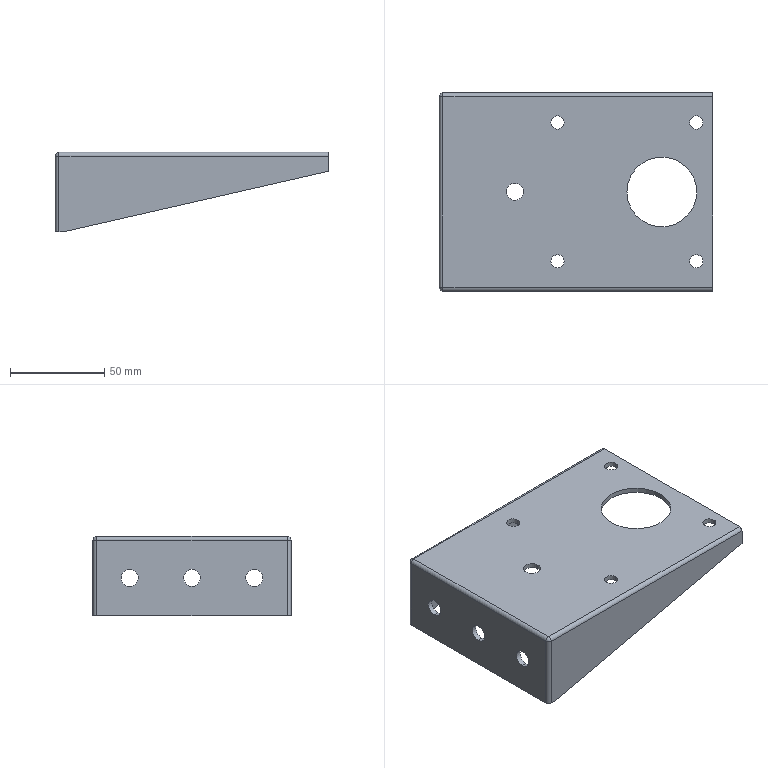Part | STEP file | 1.6米马达罩 | 1 solid | 40 faces | box 145 x 105 x 42 mm | volume 63685 mm3 | cylinder 26 | plane 12 | sphere 2 | commonest cylinder face diameters 7 x8 9 x8 4 x5 2 x3 37 x2
STEP:
#1=CARTESIAN_POINT('',(66.23,89.27,-2.6));
#2=VERTEX_POINT('',#1);
#3=CARTESIAN_POINT('',(59.23,89.27,-2.6));
#4=VERTEX_POINT('',#3);
#5=CARTESIAN_POINT('',(62.73,89.27,-2.6));
#6=DIRECTION('',(0.,0.,-1.));
#7=DIRECTION('',(-1.,0.,0.));
#8=AXIS2_PLACEMENT_3D('',#5,#6,#7);
#9=CIRCLE('',#8,3.5);
#10=EDGE_CURVE('',#2,#4,#9,.T.);
#11=ORIENTED_EDGE('',*,*,#10,.T.);
#12=CARTESIAN_POINT('',(59.23,89.27,0.));
#13=VERTEX_POINT('',#12);
#14=CARTESIAN_POINT('',(59.23,89.27,-10.));
#15=DIRECTION('',(0.,0.,1.));
#16=VECTOR('',#15,1000.);
#17=LINE('',#14,#16);
#18=EDGE_CURVE('',#4,#13,#17,.T.);
#19=ORIENTED_EDGE('',*,*,#18,.T.);
#20=CARTESIAN_POINT('',(66.23,89.27,0.));
#21=VERTEX_POINT('',#20);
#22=CARTESIAN_POINT('',(62.73,89.27,0.));
#23=DIRECTION('',(0.,0.,1.));
#24=DIRECTION('',(1.,0.,0.));
#25=AXIS2_PLACEMENT_3D('',#22,#23,#24);
#26=CIRCLE('',#25,3.5);
#27=EDGE_CURVE('',#13,#21,#26,.T.);
#28=ORIENTED_EDGE('',*,*,#27,.T.);
#29=CARTESIAN_POINT('',(66.23,89.27,-10.));
#30=DIRECTION('',(0.,0.,1.));
#31=VECTOR('',#30,1000.);
#32=LINE('',#29,#31);
#33=EDGE_CURVE('',#2,#21,#32,.T.);
#34=ORIENTED_EDGE('',*,*,#33,.F.);
#35=EDGE_LOOP('',(#11,#19,#28,#34));
#36=FACE_OUTER_BOUND('',#35,.T.);
#37=CARTESIAN_POINT('',(62.73,89.27,-10.));
#38=DIRECTION('',(0.,0.,1.));
#39=DIRECTION('',(1.,0.,0.));
#40=AXIS2_PLACEMENT_3D('',#37,#38,#39);
#41=CYLINDRICAL_SURFACE('',#40,3.5);
#42=ADVANCED_FACE('',(#36),#41,.F.);
#43=CARTESIAN_POINT('',(66.23,15.73,-2.6));
#44=VERTEX_POINT('',#43);
#45=CARTESIAN_POINT('',(59.23,15.73,-2.6));
#46=VERTEX_POINT('',#45);
#47=CARTESIAN_POINT('',(62.73,15.73,-2.6));
#48=DIRECTION('',(0.,0.,-1.));
#49=DIRECTION('',(-1.,0.,0.));
#50=AXIS2_PLACEMENT_3D('',#47,#48,#49);
#51=CIRCLE('',#50,3.5);
#52=EDGE_CURVE('',#44,#46,#51,.T.);
#53=ORIENTED_EDGE('',*,*,#52,.T.);
#54=CARTESIAN_POINT('',(59.23,15.73,0.));
#55=VERTEX_POINT('',#54);
#56=CARTESIAN_POINT('',(59.23,15.73,-10.));
#57=DIRECTION('',(0.,0.,1.));
#58=VECTOR('',#57,1000.);
#59=LINE('',#56,#58);
#60=EDGE_CURVE('',#46,#55,#59,.T.);
#61=ORIENTED_EDGE('',*,*,#60,.T.);
#62=CARTESIAN_POINT('',(66.23,15.73,0.));
#63=VERTEX_POINT('',#62);
#64=CARTESIAN_POINT('',(62.73,15.73,0.));
#65=DIRECTION('',(0.,0.,1.));
#66=DIRECTION('',(1.,0.,0.));
#67=AXIS2_PLACEMENT_3D('',#64,#65,#66);
#68=CIRCLE('',#67,3.5);
#69=EDGE_CURVE('',#55,#63,#68,.T.);
#70=ORIENTED_EDGE('',*,*,#69,.T.);
#71=CARTESIAN_POINT('',(66.23,15.73,-10.));
#72=DIRECTION('',(0.,0.,1.));
#73=VECTOR('',#72,1000.);
#74=LINE('',#71,#73);
#75=EDGE_CURVE('',#44,#63,#74,.T.);
#76=ORIENTED_EDGE('',*,*,#75,.F.);
#77=EDGE_LOOP('',(#53,#61,#70,#76));
#78=FACE_OUTER_BOUND('',#77,.T.);
#79=CARTESIAN_POINT('',(62.73,15.73,-10.));
#80=DIRECTION('',(0.,0.,1.));
#81=DIRECTION('',(1.,0.,0.));
#82=AXIS2_PLACEMENT_3D('',#79,#80,#81);
#83=CYLINDRICAL_SURFACE('',#82,3.5);
#84=ADVANCED_FACE('',(#78),#83,.F.);
#85=CARTESIAN_POINT('',(139.77,15.73,-2.6));
#86=VERTEX_POINT('',#85);
#87=CARTESIAN_POINT('',(132.77,15.73,-2.6));
#88=VERTEX_POINT('',#87);
#89=CARTESIAN_POINT('',(136.27,15.73,-2.6));
#90=DIRECTION('',(0.,0.,-1.));
#91=DIRECTION('',(-1.,0.,0.));
#92=AXIS2_PLACEMENT_3D('',#89,#90,#91);
#93=CIRCLE('',#92,3.5);
#94=EDGE_CURVE('',#86,#88,#93,.T.);
#95=ORIENTED_EDGE('',*,*,#94,.T.);
#96=CARTESIAN_POINT('',(132.77,15.73,0.));
#97=VERTEX_POINT('',#96);
#98=CARTESIAN_POINT('',(132.77,15.73,-10.));
#99=DIRECTION('',(0.,0.,1.));
#100=VECTOR('',#99,1000.);
#101=LINE('',#98,#100);
#102=EDGE_CURVE('',#88,#97,#101,.T.);
#103=ORIENTED_EDGE('',*,*,#102,.T.);
#104=CARTESIAN_POINT('',(139.77,15.73,0.));
#105=VERTEX_POINT('',#104);
#106=CARTESIAN_POINT('',(136.27,15.73,0.));
#107=DIRECTION('',(0.,0.,1.));
#108=DIRECTION('',(1.,0.,0.));
#109=AXIS2_PLACEMENT_3D('',#106,#107,#108);
#110=CIRCLE('',#109,3.5);
#111=EDGE_CURVE('',#97,#105,#110,.T.);
#112=ORIENTED_EDGE('',*,*,#111,.T.);
#113=CARTESIAN_POINT('',(139.77,15.73,-10.));
#114=DIRECTION('',(0.,0.,1.));
#115=VECTOR('',#114,1000.);
#116=LINE('',#113,#115);
#117=EDGE_CURVE('',#86,#105,#116,.T.);
#118=ORIENTED_EDGE('',*,*,#117,.F.);
#119=EDGE_LOOP('',(#95,#103,#112,#118));
#120=FACE_OUTER_BOUND('',#119,.T.);
#121=CARTESIAN_POINT('',(136.27,15.73,-10.));
#122=DIRECTION('',(0.,0.,1.));
#123=DIRECTION('',(1.,0.,0.));
#124=AXIS2_PLACEMENT_3D('',#121,#122,#123);
#125=CYLINDRICAL_SURFACE('',#124,3.5);
#126=ADVANCED_FACE('',(#120),#125,.F.);
#127=CARTESIAN_POINT('',(44.6,52.5,-2.6));
#128=VERTEX_POINT('',#127);
#129=CARTESIAN_POINT('',(35.6,52.5,-2.6));
#130=VERTEX_POINT('',#129);
#131=CARTESIAN_POINT('',(40.1,52.5,-2.6));
#132=DIRECTION('',(0.,0.,-1.));
#133=DIRECTION('',(-1.,0.,0.));
#134=AXIS2_PLACEMENT_3D('',#131,#132,#133);
#135=CIRCLE('',#134,4.5);
#136=EDGE_CURVE('',#128,#130,#135,.T.);
#137=ORIENTED_EDGE('',*,*,#136,.T.);
#138=CARTESIAN_POINT('',(35.6,52.5,0.));
#139=VERTEX_POINT('',#138);
#140=CARTESIAN_POINT('',(35.6,52.5,-10.));
#141=DIRECTION('',(0.,0.,1.));
#142=VECTOR('',#141,1000.);
#143=LINE('',#140,#142);
#144=EDGE_CURVE('',#130,#139,#143,.T.);
#145=ORIENTED_EDGE('',*,*,#144,.T.);
#146=CARTESIAN_POINT('',(44.6,52.5,0.));
#147=VERTEX_POINT('',#146);
#148=CARTESIAN_POINT('',(40.1,52.5,0.));
#149=DIRECTION('',(0.,0.,1.));
#150=DIRECTION('',(1.,0.,0.));
#151=AXIS2_PLACEMENT_3D('',#148,#149,#150);
#152=CIRCLE('',#151,4.5);
#153=EDGE_CURVE('',#139,#147,#152,.T.);
#154=ORIENTED_EDGE('',*,*,#153,.T.);
#155=CARTESIAN_POINT('',(44.6,52.5,-10.));
#156=DIRECTION('',(0.,0.,1.));
#157=VECTOR('',#156,1000.);
#158=LINE('',#155,#157);
#159=EDGE_CURVE('',#128,#147,#158,.T.);
#160=ORIENTED_EDGE('',*,*,#159,.F.);
#161=EDGE_LOOP('',(#137,#145,#154,#160));
#162=FACE_OUTER_BOUND('',#161,.T.);
#163=CARTESIAN_POINT('',(40.1,52.5,-10.));
#164=DIRECTION('',(0.,0.,1.));
#165=DIRECTION('',(1.,0.,0.));
#166=AXIS2_PLACEMENT_3D('',#163,#164,#165);
#167=CYLINDRICAL_SURFACE('',#166,4.5);
#168=ADVANCED_FACE('',(#162),#167,.F.);
#169=CARTESIAN_POINT('',(139.77,89.27,-2.6));
#170=VERTEX_POINT('',#169);
#171=CARTESIAN_POINT('',(132.77,89.27,-2.6));
#172=VERTEX_POINT('',#171);
#173=CARTESIAN_POINT('',(136.27,89.27,-2.6));
#174=DIRECTION('',(0.,0.,-1.));
#175=DIRECTION('',(-1.,0.,0.));
#176=AXIS2_PLACEMENT_3D('',#173,#174,#175);
#177=CIRCLE('',#176,3.5);
#178=EDGE_CURVE('',#170,#172,#177,.T.);
#179=ORIENTED_EDGE('',*,*,#178,.T.);
#180=CARTESIAN_POINT('',(132.77,89.27,0.));
#181=VERTEX_POINT('',#180);
#182=CARTESIAN_POINT('',(132.77,89.27,-10.));
#183=DIRECTION('',(0.,0.,1.));
#184=VECTOR('',#183,1000.);
#185=LINE('',#182,#184);
#186=EDGE_CURVE('',#172,#181,#185,.T.);
#187=ORIENTED_EDGE('',*,*,#186,.T.);
#188=CARTESIAN_POINT('',(139.77,89.27,0.));
#189=VERTEX_POINT('',#188);
#190=CARTESIAN_POINT('',(136.27,89.27,0.));
#191=DIRECTION('',(0.,0.,1.));
#192=DIRECTION('',(1.,0.,0.));
#193=AXIS2_PLACEMENT_3D('',#190,#191,#192);
#194=CIRCLE('',#193,3.5);
#195=EDGE_CURVE('',#181,#189,#194,.T.);
#196=ORIENTED_EDGE('',*,*,#195,.T.);
#197=CARTESIAN_POINT('',(139.77,89.27,-10.));
#198=DIRECTION('',(0.,0.,1.));
#199=VECTOR('',#198,1000.);
#200=LINE('',#197,#199);
#201=EDGE_CURVE('',#170,#189,#200,.T.);
#202=ORIENTED_EDGE('',*,*,#201,.F.);
#203=EDGE_LOOP('',(#179,#187,#196,#202));
#204=FACE_OUTER_BOUND('',#203,.T.);
#205=CARTESIAN_POINT('',(136.27,89.27,-10.));
#206=DIRECTION('',(0.,0.,1.));
#207=DIRECTION('',(1.,0.,0.));
#208=AXIS2_PLACEMENT_3D('',#205,#206,#207);
#209=CYLINDRICAL_SURFACE('',#208,3.5);
#210=ADVANCED_FACE('',(#204),#209,.F.);
#211=CARTESIAN_POINT('',(136.5,52.5,-2.6));
#212=VERTEX_POINT('',#211);
#213=CARTESIAN_POINT('',(99.5,52.5,-2.6));
#214=VERTEX_POINT('',#213);
#215=CARTESIAN_POINT('',(118.,52.5,-2.6));
#216=DIRECTION('',(0.,0.,-1.));
#217=DIRECTION('',(-1.,0.,0.));
#218=AXIS2_PLACEMENT_3D('',#215,#216,#217);
#219=CIRCLE('',#218,18.5);
#220=EDGE_CURVE('',#212,#214,#219,.T.);
#221=ORIENTED_EDGE('',*,*,#220,.T.);
#222=CARTESIAN_POINT('',(99.5,52.5,0.));
#223=VERTEX_POINT('',#222);
#224=CARTESIAN_POINT('',(99.5,52.5,-10.));
#225=DIRECTION('',(0.,0.,1.));
#226=VECTOR('',#225,1000.);
#227=LINE('',#224,#226);
#228=EDGE_CURVE('',#214,#223,#227,.T.);
#229=ORIENTED_EDGE('',*,*,#228,.T.);
#230=CARTESIAN_POINT('',(136.5,52.5,0.));
#231=VERTEX_POINT('',#230);
#232=CARTESIAN_POINT('',(118.,52.5,0.));
#233=DIRECTION('',(0.,0.,1.));
#234=DIRECTION('',(1.,0.,0.));
#235=AXIS2_PLACEMENT_3D('',#232,#233,#234);
#236=CIRCLE('',#235,18.5);
#237=EDGE_CURVE('',#223,#231,#236,.T.);
#238=ORIENTED_EDGE('',*,*,#237,.T.);
#239=CARTESIAN_POINT('',(136.5,52.5,-10.));
#240=DIRECTION('',(0.,0.,1.));
#241=VECTOR('',#240,1000.);
#242=LINE('',#239,#241);
#243=EDGE_CURVE('',#212,#231,#242,.T.);
#244=ORIENTED_EDGE('',*,*,#243,.F.);
#245=EDGE_LOOP('',(#221,#229,#238,#244));
#246=FACE_OUTER_BOUND('',#245,.T.);
#247=CARTESIAN_POINT('',(118.,52.5,-10.));
#248=DIRECTION('',(0.,0.,1.));
#249=DIRECTION('',(1.,0.,0.));
#250=AXIS2_PLACEMENT_3D('',#247,#248,#249);
#251=CYLINDRICAL_SURFACE('',#250,18.5);
#252=ADVANCED_FACE('',(#246),#251,.F.);
#253=CARTESIAN_POINT('',(2.6,19.5,-17.5));
#254=VERTEX_POINT('',#253);
#255=CARTESIAN_POINT('',(2.6,19.5,-26.5));
#256=VERTEX_POINT('',#255);
#257=CARTESIAN_POINT('',(2.6,19.5,-22.));
#258=DIRECTION('',(1.,0.,0.));
#259=DIRECTION('',(0.,0.,-1.));
#260=AXIS2_PLACEMENT_3D('',#257,#258,#259);
#261=CIRCLE('',#260,4.5);
#262=EDGE_CURVE('',#254,#256,#261,.T.);
#263=ORIENTED_EDGE('',*,*,#262,.T.);
#264=CARTESIAN_POINT('',(0.,19.5,-26.5));
#265=VERTEX_POINT('',#264);
#266=CARTESIAN_POINT('',(10.,19.5,-26.5));
#267=DIRECTION('',(-1.,0.,0.));
#268=VECTOR('',#267,1000.);
#269=LINE('',#266,#268);
#270=EDGE_CURVE('',#256,#265,#269,.T.);
#271=ORIENTED_EDGE('',*,*,#270,.T.);
#272=CARTESIAN_POINT('',(0.,19.5,-17.5));
#273=VERTEX_POINT('',#272);
#274=CARTESIAN_POINT('',(0.,19.5,-22.));
#275=DIRECTION('',(-1.,0.,0.));
#276=DIRECTION('',(0.,0.,1.));
#277=AXIS2_PLACEMENT_3D('',#274,#275,#276);
#278=CIRCLE('',#277,4.5);
#279=EDGE_CURVE('',#265,#273,#278,.T.);
#280=ORIENTED_EDGE('',*,*,#279,.T.);
#281=CARTESIAN_POINT('',(10.,19.5,-17.5));
#282=DIRECTION('',(-1.,0.,0.));
#283=VECTOR('',#282,1000.);
#284=LINE('',#281,#283);
#285=EDGE_CURVE('',#254,#273,#284,.T.);
#286=ORIENTED_EDGE('',*,*,#285,.F.);
#287=EDGE_LOOP('',(#263,#271,#280,#286));
#288=FACE_OUTER_BOUND('',#287,.T.);
#289=CARTESIAN_POINT('',(10.,19.5,-22.));
#290=DIRECTION('',(-1.,0.,0.));
#291=DIRECTION('',(0.,0.,1.));
#292=AXIS2_PLACEMENT_3D('',#289,#290,#291);
#293=CYLINDRICAL_SURFACE('',#292,4.5);
#294=ADVANCED_FACE('',(#288),#293,.F.);
#295=CARTESIAN_POINT('',(2.6,85.5,-17.5));
#296=VERTEX_POINT('',#295);
#297=CARTESIAN_POINT('',(2.6,85.5,-26.5));
#298=VERTEX_POINT('',#297);
#299=CARTESIAN_POINT('',(2.6,85.5,-22.));
#300=DIRECTION('',(1.,0.,0.));
#301=DIRECTION('',(0.,0.,-1.));
#302=AXIS2_PLACEMENT_3D('',#299,#300,#301);
#303=CIRCLE('',#302,4.5);
#304=EDGE_CURVE('',#296,#298,#303,.T.);
#305=ORIENTED_EDGE('',*,*,#304,.T.);
#306=CARTESIAN_POINT('',(0.,85.5,-26.5));
#307=VERTEX_POINT('',#306);
#308=CARTESIAN_POINT('',(10.,85.5,-26.5));
#309=DIRECTION('',(-1.,0.,0.));
#310=VECTOR('',#309,1000.);
#311=LINE('',#308,#310);
#312=EDGE_CURVE('',#298,#307,#311,.T.);
#313=ORIENTED_EDGE('',*,*,#312,.T.);
#314=CARTESIAN_POINT('',(0.,85.5,-17.5));
#315=VERTEX_POINT('',#314);
#316=CARTESIAN_POINT('',(0.,85.5,-22.));
#317=DIRECTION('',(-1.,0.,0.));
#318=DIRECTION('',(0.,0.,1.));
#319=AXIS2_PLACEMENT_3D('',#316,#317,#318);
#320=CIRCLE('',#319,4.5);
#321=EDGE_CURVE('',#307,#315,#320,.T.);
#322=ORIENTED_EDGE('',*,*,#321,.T.);
#323=CARTESIAN_POINT('',(10.,85.5,-17.5));
#324=DIRECTION('',(-1.,0.,0.));
#325=VECTOR('',#324,1000.);
#326=LINE('',#323,#325);
#327=EDGE_CURVE('',#296,#315,#326,.T.);
#328=ORIENTED_EDGE('',*,*,#327,.F.);
#329=EDGE_LOOP('',(#305,#313,#322,#328));
#330=FACE_OUTER_BOUND('',#329,.T.);
#331=CARTESIAN_POINT('',(10.,85.5,-22.));
#332=DIRECTION('',(-1.,0.,0.));
#333=DIRECTION('',(0.,0.,1.));
#334=AXIS2_PLACEMENT_3D('',#331,#332,#333);
#335=CYLINDRICAL_SURFACE('',#334,4.5);
#336=ADVANCED_FACE('',(#330),#335,.F.);
#337=CARTESIAN_POINT('',(2.6,52.5,-17.5));
#338=VERTEX_POINT('',#337);
#339=CARTESIAN_POINT('',(2.6,52.5,-26.5));
#340=VERTEX_POINT('',#339);
#341=CARTESIAN_POINT('',(2.6,52.5,-22.));
#342=DIRECTION('',(1.,0.,0.));
#343=DIRECTION('',(0.,0.,-1.));
#344=AXIS2_PLACEMENT_3D('',#341,#342,#343);
#345=CIRCLE('',#344,4.5);
#346=EDGE_CURVE('',#338,#340,#345,.T.);
#347=ORIENTED_EDGE('',*,*,#346,.T.);
#348=CARTESIAN_POINT('',(0.,52.5,-26.5));
#349=VERTEX_POINT('',#348);
#350=CARTESIAN_POINT('',(10.,52.5,-26.5));
#351=DIRECTION('',(-1.,0.,0.));
#352=VECTOR('',#351,1000.);
#353=LINE('',#350,#352);
#354=EDGE_CURVE('',#340,#349,#353,.T.);
#355=ORIENTED_EDGE('',*,*,#354,.T.);
#356=CARTESIAN_POINT('',(0.,52.5,-17.5));
#357=VERTEX_POINT('',#356);
#358=CARTESIAN_POINT('',(0.,52.5,-22.));
#359=DIRECTION('',(-1.,0.,0.));
#360=DIRECTION('',(0.,0.,1.));
#361=AXIS2_PLACEMENT_3D('',#358,#359,#360);
#362=CIRCLE('',#361,4.5);
#363=EDGE_CURVE('',#349,#357,#362,.T.);
#364=ORIENTED_EDGE('',*,*,#363,.T.);
#365=CARTESIAN_POINT('',(10.,52.5,-17.5));
#366=DIRECTION('',(-1.,0.,0.));
#367=VECTOR('',#366,1000.);
#368=LINE('',#365,#367);
#369=EDGE_CURVE('',#338,#357,#368,.T.);
#370=ORIENTED_EDGE('',*,*,#369,.F.);
#371=EDGE_LOOP('',(#347,#355,#364,#370));
#372=FACE_OUTER_BOUND('',#371,.T.);
#373=CARTESIAN_POINT('',(10.,52.5,-22.));
#374=DIRECTION('',(-1.,0.,0.));
#375=DIRECTION('',(0.,0.,1.));
#376=AXIS2_PLACEMENT_3D('',#373,#374,#375);
#377=CYLINDRICAL_SURFACE('',#376,4.5);
#378=ADVANCED_FACE('',(#372),#377,.F.);
#379=CARTESIAN_POINT('',(145.,103.,0.));
#380=VERTEX_POINT('',#379);
#381=CARTESIAN_POINT('',(145.,2.,0.));
#382=VERTEX_POINT('',#381);
#383=CARTESIAN_POINT('',(145.,105.,0.));
#384=DIRECTION('',(0.,-1.,0.));
#385=VECTOR('',#384,1000.);
#386=LINE('',#383,#385);
#387=EDGE_CURVE('',#380,#382,#386,.T.);
#388=ORIENTED_EDGE('',*,*,#387,.T.);
#389=CARTESIAN_POINT('',(145.,0.,-2.));
#390=VERTEX_POINT('',#389);
#391=CARTESIAN_POINT('',(145.,2.,-2.));
#392=DIRECTION('',(1.,0.,0.));
#393=DIRECTION('',(0.,0.,1.));
#394=AXIS2_PLACEMENT_3D('',#391,#392,#393);
#395=CIRCLE('',#394,2.);
#396=EDGE_CURVE('',#382,#390,#395,.T.);
#397=ORIENTED_EDGE('',*,*,#396,.T.);
#398=CARTESIAN_POINT('',(145.,0.,-10.));
#399=VERTEX_POINT('',#398);
#400=CARTESIAN_POINT('',(145.,0.,-10.));
#401=DIRECTION('',(0.,0.,-1.));
#402=VECTOR('',#401,1000.);
#403=LINE('',#400,#402);
#404=EDGE_CURVE('',#390,#399,#403,.T.);
#405=ORIENTED_EDGE('',*,*,#404,.T.);
#406=CARTESIAN_POINT('',(145.,2.6,-10.));
#407=VERTEX_POINT('',#406);
#408=CARTESIAN_POINT('',(145.,105.,-10.));
#409=DIRECTION('',(0.,-1.,0.));
#410=VECTOR('',#409,1000.);
#411=LINE('',#408,#410);
#412=EDGE_CURVE('',#407,#399,#411,.T.);
#413=ORIENTED_EDGE('',*,*,#412,.F.);
#414=CARTESIAN_POINT('',(145.,2.6,-3.6));
#415=VERTEX_POINT('',#414);
#416=CARTESIAN_POINT('',(145.,2.6,0.));
#417=DIRECTION('',(0.,0.,-1.));
#418=VECTOR('',#417,1000.);
#419=LINE('',#416,#418);
#420=EDGE_CURVE('',#415,#407,#419,.T.);
#421=ORIENTED_EDGE('',*,*,#420,.F.);
#422=CARTESIAN_POINT('',(145.,3.6,-2.6));
#423=VERTEX_POINT('',#422);
#424=CARTESIAN_POINT('',(145.,3.6,-3.6));
#425=DIRECTION('',(-1.,0.,0.));
#426=DIRECTION('',(0.,0.,1.));
#427=AXIS2_PLACEMENT_3D('',#424,#425,#426);
#428=CIRCLE('',#427,1.);
#429=EDGE_CURVE('',#415,#423,#428,.T.);
#430=ORIENTED_EDGE('',*,*,#429,.T.);
#431=CARTESIAN_POINT('',(145.,101.4,-2.6));
#432=VERTEX_POINT('',#431);
#433=CARTESIAN_POINT('',(145.,105.,-2.6));
#434=DIRECTION('',(0.,-1.,0.));
#435=VECTOR('',#434,1000.);
#436=LINE('',#433,#435);
#437=EDGE_CURVE('',#432,#423,#436,.T.);
#438=ORIENTED_EDGE('',*,*,#437,.F.);
#439=CARTESIAN_POINT('',(145.,102.4,-3.6));
#440=VERTEX_POINT('',#439);
#441=CARTESIAN_POINT('',(145.,101.4,-3.6));
#442=DIRECTION('',(-1.,0.,0.));
#443=DIRECTION('',(0.,0.,1.));
#444=AXIS2_PLACEMENT_3D('',#441,#442,#443);
#445=CIRCLE('',#444,1.);
#446=EDGE_CURVE('',#432,#440,#445,.T.);
#447=ORIENTED_EDGE('',*,*,#446,.T.);
#448=CARTESIAN_POINT('',(145.,102.4,-10.));
#449=VERTEX_POINT('',#448);
#450=CARTESIAN_POINT('',(145.,102.4,0.));
#451=DIRECTION('',(0.,0.,-1.));
#452=VECTOR('',#451,1000.);
#453=LINE('',#450,#452);
#454=EDGE_CURVE('',#440,#449,#453,.T.);
#455=ORIENTED_EDGE('',*,*,#454,.T.);
#456=CARTESIAN_POINT('',(145.,105.,-10.));
#457=VERTEX_POINT('',#456);
#458=CARTESIAN_POINT('',(145.,105.,-10.));
#459=DIRECTION('',(0.,-1.,0.));
#460=VECTOR('',#459,1000.);
#461=LINE('',#458,#460);
#462=EDGE_CURVE('',#457,#449,#461,.T.);
#463=ORIENTED_EDGE('',*,*,#462,.F.);
#464=CARTESIAN_POINT('',(145.,105.,-2.));
#465=VERTEX_POINT('',#464);
#466=CARTESIAN_POINT('',(145.,105.,-10.));
#467=DIRECTION('',(0.,0.,-1.));
#468=VECTOR('',#467,1000.);
#469=LINE('',#466,#468);
#470=EDGE_CURVE('',#465,#457,#469,.T.);
#471=ORIENTED_EDGE('',*,*,#470,.F.);
#472=CARTESIAN_POINT('',(145.,103.,-2.));
#473=DIRECTION('',(1.,0.,0.));
#474=DIRECTION('',(0.,0.,1.));
#475=AXIS2_PLACEMENT_3D('',#472,#473,#474);
#476=CIRCLE('',#475,2.);
#477=EDGE_CURVE('',#465,#380,#476,.T.);
#478=ORIENTED_EDGE('',*,*,#477,.T.);
#479=EDGE_LOOP('',(#388,#397,#405,#413,#421,#430,#438,#447,#455,#463,#471,#478));
#480=FACE_OUTER_BOUND('',#479,.T.);
#481=CARTESIAN_POINT('',(145.,105.,-10.));
#482=DIRECTION('',(-1.,0.,0.));
#483=DIRECTION('',(0.,0.,1.));
#484=AXIS2_PLACEMENT_3D('',#481,#482,#483);
#485=PLANE('',#484);
#486=ADVANCED_FACE('',(#480),#485,.F.);
#487=CARTESIAN_POINT('',(5.,2.6,-42.));
#488=VERTEX_POINT('',#487);
#489=CARTESIAN_POINT('',(9.372,2.6,-41.001));
#490=DIRECTION('',(-0.9749,0.,-0.2228));
#491=VECTOR('',#490,1000.);
#492=LINE('',#489,#491);
#493=EDGE_CURVE('',#407,#488,#492,.T.);
#494=ORIENTED_EDGE('',*,*,#493,.F.);
#495=ORIENTED_EDGE('',*,*,#412,.T.);
#496=CARTESIAN_POINT('',(5.,0.,-42.));
#497=VERTEX_POINT('',#496);
#498=CARTESIAN_POINT('',(5.,0.,-42.));
#499=DIRECTION('',(-0.9749,0.,-0.2228));
#500=VECTOR('',#499,1000.);
#501=LINE('',#498,#500);
#502=EDGE_CURVE('',#399,#497,#501,.T.);
#503=ORIENTED_EDGE('',*,*,#502,.T.);
#504=CARTESIAN_POINT('',(5.,105.,-42.));
#505=DIRECTION('',(0.,-1.,0.));
#506=VECTOR('',#505,1000.);
#507=LINE('',#504,#506);
#508=EDGE_CURVE('',#488,#497,#507,.T.);
#509=ORIENTED_EDGE('',*,*,#508,.F.);
#510=EDGE_LOOP('',(#494,#495,#503,#509));
#511=FACE_OUTER_BOUND('',#510,.T.);
#512=CARTESIAN_POINT('',(5.,105.,-42.));
#513=DIRECTION('',(-0.2228,0.,0.9749));
#514=DIRECTION('',(0.9749,0.,0.2228));
#515=AXIS2_PLACEMENT_3D('',#512,#513,#514);
#516=PLANE('',#515);
#517=ADVANCED_FACE('',(#511),#516,.F.);
#518=CARTESIAN_POINT('',(2.,0.,-42.));
#519=VERTEX_POINT('',#518);
#520=CARTESIAN_POINT('',(0.,0.,-42.));
#521=DIRECTION('',(-1.,0.,0.));
#522=VECTOR('',#521,1000.);
#523=LINE('',#520,#522);
#524=EDGE_CURVE('',#497,#519,#523,.T.);
#525=ORIENTED_EDGE('',*,*,#524,.T.);
#526=CARTESIAN_POINT('',(0.,2.,-42.));
#527=VERTEX_POINT('',#526);
#528=CARTESIAN_POINT('',(2.,2.,-42.));
#529=DIRECTION('',(0.,0.,-1.));
#530=DIRECTION('',(1.,0.,0.));
#531=AXIS2_PLACEMENT_3D('',#528,#529,#530);
#532=CIRCLE('',#531,2.);
#533=EDGE_CURVE('',#519,#527,#532,.T.);
#534=ORIENTED_EDGE('',*,*,#533,.T.);
#535=CARTESIAN_POINT('',(0.,103.,-42.));
#536=VERTEX_POINT('',#535);
#537=CARTESIAN_POINT('',(0.,105.,-42.));
#538=DIRECTION('',(0.,-1.,0.));
#539=VECTOR('',#538,1000.);
#540=LINE('',#537,#539);
#541=EDGE_CURVE('',#536,#527,#540,.T.);
#542=ORIENTED_EDGE('',*,*,#541,.F.);
#543=CARTESIAN_POINT('',(2.,105.,-42.));
#544=VERTEX_POINT('',#543);
#545=CARTESIAN_POINT('',(2.,103.,-42.));
#546=DIRECTION('',(0.,0.,-1.));
#547=DIRECTION('',(1.,0.,0.));
#548=AXIS2_PLACEMENT_3D('',#545,#546,#547);
#549=CIRCLE('',#548,2.);
#550=EDGE_CURVE('',#536,#544,#549,.T.);
#551=ORIENTED_EDGE('',*,*,#550,.T.);
#552=CARTESIAN_POINT('',(5.,105.,-42.));
#553=VERTEX_POINT('',#552);
#554=CARTESIAN_POINT('',(0.,105.,-42.));
#555=DIRECTION('',(-1.,0.,0.));
#556=VECTOR('',#555,1000.);
#557=LINE('',#554,#556);
#558=EDGE_CURVE('',#553,#544,#557,.T.);
#559=ORIENTED_EDGE('',*,*,#558,.F.);
#560=CARTESIAN_POINT('',(5.,102.4,-42.));
#561=VERTEX_POINT('',#560);
#562=CARTESIAN_POINT('',(5.,105.,-42.));
#563=DIRECTION('',(0.,-1.,0.));
#564=VECTOR('',#563,1000.);
#565=LINE('',#562,#564);
#566=EDGE_CURVE('',#553,#561,#565,.T.);
#567=ORIENTED_EDGE('',*,*,#566,.T.);
#568=CARTESIAN_POINT('',(2.6,102.4,-42.));
#569=VERTEX_POINT('',#568);
#570=CARTESIAN_POINT('',(0.,102.4,-42.));
#571=DIRECTION('',(-1.,0.,0.));
#572=VECTOR('',#571,1000.);
#573=LINE('',#570,#572);
#574=EDGE_CURVE('',#561,#569,#573,.T.);
#575=ORIENTED_EDGE('',*,*,#574,.T.);
#576=CARTESIAN_POINT('',(2.6,2.6,-42.));
#577=VERTEX_POINT('',#576);
#578=CARTESIAN_POINT('',(2.6,105.,-42.));
#579=DIRECTION('',(0.,-1.,0.));
#580=VECTOR('',#579,1000.);
#581=LINE('',#578,#580);
#582=EDGE_CURVE('',#569,#577,#581,.T.);
#583=ORIENTED_EDGE('',*,*,#582,.T.);
#584=CARTESIAN_POINT('',(0.,2.6,-42.));
#585=DIRECTION('',(-1.,0.,0.));
#586=VECTOR('',#585,1000.);
#587=LINE('',#584,#586);
#588=EDGE_CURVE('',#488,#577,#587,.T.);
#589=ORIENTED_EDGE('',*,*,#588,.F.);
#590=ORIENTED_EDGE('',*,*,#508,.T.);
#591=EDGE_LOOP('',(#525,#534,#542,#551,#559,#567,#575,#583,#589,#590));
#592=FACE_OUTER_BOUND('',#591,.T.);
#593=CARTESIAN_POINT('',(0.,105.,-42.));
#594=DIRECTION('',(0.,0.,1.));
#595=DIRECTION('',(1.,0.,0.));
#596=AXIS2_PLACEMENT_3D('',#593,#594,#595);
#597=PLANE('',#596);
#598=ADVANCED_FACE('',(#592),#597,.F.);
#599=CARTESIAN_POINT('',(62.73,89.27,0.));
#600=DIRECTION('',(0.,0.,1.));
#601=DIRECTION('',(1.,0.,0.));
#602=AXIS2_PLACEMENT_3D('',#599,#600,#601);
#603=CIRCLE('',#602,3.5);
#604=EDGE_CURVE('',#21,#13,#603,.T.);
#605=ORIENTED_EDGE('',*,*,#604,.F.);
#606=ORIENTED_EDGE('',*,*,#27,.F.);
#607=EDGE_LOOP('',(#605,#606));
#608=FACE_BOUND('',#607,.T.);
#609=CARTESIAN_POINT('',(62.73,15.73,0.));
#610=DIRECTION('',(0.,0.,1.));
#611=DIRECTION('',(1.,0.,0.));
#612=AXIS2_PLACEMENT_3D('',#609,#610,#611);
#613=CIRCLE('',#612,3.5);
#614=EDGE_CURVE('',#63,#55,#613,.T.);
#615=ORIENTED_EDGE('',*,*,#614,.F.);
#616=ORIENTED_EDGE('',*,*,#69,.F.);
#617=EDGE_LOOP('',(#615,#616));
#618=FACE_BOUND('',#617,.T.);
#619=CARTESIAN_POINT('',(136.27,15.73,0.));
#620=DIRECTION('',(0.,0.,1.));
#621=DIRECTION('',(1.,0.,0.));
#622=AXIS2_PLACEMENT_3D('',#619,#620,#621);
#623=CIRCLE('',#622,3.5);
#624=EDGE_CURVE('',#105,#97,#623,.T.);
#625=ORIENTED_EDGE('',*,*,#624,.F.);
#626=ORIENTED_EDGE('',*,*,#111,.F.);
#627=EDGE_LOOP('',(#625,#626));
#628=FACE_BOUND('',#627,.T.);
#629=CARTESIAN_POINT('',(40.1,52.5,0.));
#630=DIRECTION('',(0.,0.,1.));
#631=DIRECTION('',(1.,0.,0.));
#632=AXIS2_PLACEMENT_3D('',#629,#630,#631);
#633=CIRCLE('',#632,4.5);
#634=EDGE_CURVE('',#147,#139,#633,.T.);
#635=ORIENTED_EDGE('',*,*,#634,.F.);
#636=ORIENTED_EDGE('',*,*,#153,.F.);
#637=EDGE_LOOP('',(#635,#636));
#638=FACE_BOUND('',#637,.T.);
#639=CARTESIAN_POINT('',(136.27,89.27,0.));
#640=DIRECTION('',(0.,0.,1.));
#641=DIRECTION('',(1.,0.,0.));
#642=AXIS2_PLACEMENT_3D('',#639,#640,#641);
#643=CIRCLE('',#642,3.5);
#644=EDGE_CURVE('',#189,#181,#643,.T.);
#645=ORIENTED_EDGE('',*,*,#644,.F.);
#646=ORIENTED_EDGE('',*,*,#195,.F.);
#647=EDGE_LOOP('',(#645,#646));
#648=FACE_BOUND('',#647,.T.);
#649=CARTESIAN_POINT('',(118.,52.5,0.));
#650=DIRECTION('',(0.,0.,1.));
#651=DIRECTION('',(1.,0.,0.));
#652=AXIS2_PLACEMENT_3D('',#649,#650,#651);
#653=CIRCLE('',#652,18.5);
#654=EDGE_CURVE('',#231,#223,#653,.T.);
#655=ORIENTED_EDGE('',*,*,#654,.F.);
#656=ORIENTED_EDGE('',*,*,#237,.F.);
#657=EDGE_LOOP('',(#655,#656));
#658=FACE_BOUND('',#657,.T.);
#659=CARTESIAN_POINT('',(2.,103.,0.));
#660=VERTEX_POINT('',#659);
#661=CARTESIAN_POINT('',(2.,2.,0.));
#662=VERTEX_POINT('',#661);
#663=CARTESIAN_POINT('',(2.,105.,0.));
#664=DIRECTION('',(0.,-1.,0.));
#665=VECTOR('',#664,1000.);
#666=LINE('',#663,#665);
#667=EDGE_CURVE('',#660,#662,#666,.T.);
#668=ORIENTED_EDGE('',*,*,#667,.T.);
#669=CARTESIAN_POINT('',(145.,2.,0.));
#670=DIRECTION('',(1.,0.,0.));
#671=VECTOR('',#670,1000.);
#672=LINE('',#669,#671);
#673=EDGE_CURVE('',#662,#382,#672,.T.);
#674=ORIENTED_EDGE('',*,*,#673,.T.);
#675=ORIENTED_EDGE('',*,*,#387,.F.);
#676=CARTESIAN_POINT('',(145.,103.,0.));
#677=DIRECTION('',(-1.,0.,0.));
#678=VECTOR('',#677,1000.);
#679=LINE('',#676,#678);
#680=EDGE_CURVE('',#380,#660,#679,.T.);
#681=ORIENTED_EDGE('',*,*,#680,.T.);
#682=EDGE_LOOP('',(#668,#674,#675,#681));
#683=FACE_OUTER_BOUND('',#682,.T.);
#684=CARTESIAN_POINT('',(145.,105.,0.));
#685=DIRECTION('',(0.,0.,-1.));
#686=DIRECTION('',(-1.,0.,0.));
#687=AXIS2_PLACEMENT_3D('',#684,#685,#686);
#688=PLANE('',#687);
#689=ADVANCED_FACE('',(#608,#618,#628,#638,#648,#658,#683),#688,.F.);
#690=ORIENTED_EDGE('',*,*,#462,.T.);
#691=CARTESIAN_POINT('',(9.372,102.4,-41.001));
#692=DIRECTION('',(-0.9749,0.,-0.2228));
#693=VECTOR('',#692,1000.);
#694=LINE('',#691,#693);
#695=EDGE_CURVE('',#449,#561,#694,.T.);
#696=ORIENTED_EDGE('',*,*,#695,.T.);
#697=ORIENTED_EDGE('',*,*,#566,.F.);
#698=CARTESIAN_POINT('',(5.,105.,-42.));
#699=DIRECTION('',(-0.9749,0.,-0.2228));
#700=VECTOR('',#699,1000.);
#701=LINE('',#698,#700);
#702=EDGE_CURVE('',#457,#553,#701,.T.);
#703=ORIENTED_EDGE('',*,*,#702,.F.);
#704=EDGE_LOOP('',(#690,#696,#697,#703));
#705=FACE_OUTER_BOUND('',#704,.T.);
#706=CARTESIAN_POINT('',(5.,105.,-42.));
#707=DIRECTION('',(-0.2228,0.,0.9749));
#708=DIRECTION('',(0.9749,0.,0.2228));
#709=AXIS2_PLACEMENT_3D('',#706,#707,#708);
#710=PLANE('',#709);
#711=ADVANCED_FACE('',(#705),#710,.F.);
#712=CARTESIAN_POINT('',(0.,19.5,-22.));
#713=DIRECTION('',(-1.,0.,0.));
#714=DIRECTION('',(0.,0.,1.));
#715=AXIS2_PLACEMENT_3D('',#712,#713,#714);
#716=CIRCLE('',#715,4.5);
#717=EDGE_CURVE('',#273,#265,#716,.T.);
#718=ORIENTED_EDGE('',*,*,#717,.F.);
#719=ORIENTED_EDGE('',*,*,#279,.F.);
#720=EDGE_LOOP('',(#718,#719));
#721=FACE_BOUND('',#720,.T.);
#722=CARTESIAN_POINT('',(0.,85.5,-22.));
#723=DIRECTION('',(-1.,0.,0.));
#724=DIRECTION('',(0.,0.,1.));
#725=AXIS2_PLACEMENT_3D('',#722,#723,#724);
#726=CIRCLE('',#725,4.5);
#727=EDGE_CURVE('',#315,#307,#726,.T.);
#728=ORIENTED_EDGE('',*,*,#727,.F.);
#729=ORIENTED_EDGE('',*,*,#321,.F.);
#730=EDGE_LOOP('',(#728,#729));
#731=FACE_BOUND('',#730,.T.);
#732=CARTESIAN_POINT('',(0.,52.5,-22.));
#733=DIRECTION('',(-1.,0.,0.));
#734=DIRECTION('',(0.,0.,1.));
#735=AXIS2_PLACEMENT_3D('',#732,#733,#734);
#736=CIRCLE('',#735,4.5);
#737=EDGE_CURVE('',#357,#349,#736,.T.);
#738=ORIENTED_EDGE('',*,*,#737,.F.);
#739=ORIENTED_EDGE('',*,*,#363,.F.);
#740=EDGE_LOOP('',(#738,#739));
#741=FACE_BOUND('',#740,.T.);
#742=ORIENTED_EDGE('',*,*,#541,.T.);
#743=CARTESIAN_POINT('',(0.,2.,-2.));
#744=VERTEX_POINT('',#743);
#745=CARTESIAN_POINT('',(0.,2.,0.));
#746=DIRECTION('',(0.,0.,1.));
#747=VECTOR('',#746,1000.);
#748=LINE('',#745,#747);
#749=EDGE_CURVE('',#527,#744,#748,.T.);
#750=ORIENTED_EDGE('',*,*,#749,.T.);
#751=CARTESIAN_POINT('',(0.,103.,-2.));
#752=VERTEX_POINT('',#751);
#753=CARTESIAN_POINT('',(0.,105.,-2.));
#754=DIRECTION('',(0.,1.,0.));
#755=VECTOR('',#754,1000.);
#756=LINE('',#753,#755);
#757=EDGE_CURVE('',#744,#752,#756,.T.);
#758=ORIENTED_EDGE('',*,*,#757,.T.);
#759=CARTESIAN_POINT('',(0.,103.,0.));
#760=DIRECTION('',(0.,0.,-1.));
#761=VECTOR('',#760,1000.);
#762=LINE('',#759,#761);
#763=EDGE_CURVE('',#752,#536,#762,.T.);
#764=ORIENTED_EDGE('',*,*,#763,.T.);
#765=EDGE_LOOP('',(#742,#750,#758,#764));
#766=FACE_OUTER_BOUND('',#765,.T.);
#767=CARTESIAN_POINT('',(0.,105.,0.));
#768=DIRECTION('',(1.,0.,0.));
#769=DIRECTION('',(0.,0.,-1.));
#770=AXIS2_PLACEMENT_3D('',#767,#768,#769);
#771=PLANE('',#770);
#772=ADVANCED_FACE('',(#721,#731,#741,#766),#771,.F.);
#773=ORIENTED_EDGE('',*,*,#558,.T.);
#774=CARTESIAN_POINT('',(2.,105.,-2.));
#775=VERTEX_POINT('',#774);
#776=CARTESIAN_POINT('',(2.,105.,0.));
#777=DIRECTION('',(0.,0.,1.));
#778=VECTOR('',#777,1000.);
#779=LINE('',#776,#778);
#780=EDGE_CURVE('',#544,#775,#779,.T.);
#781=ORIENTED_EDGE('',*,*,#780,.T.);
#782=CARTESIAN_POINT('',(0.,105.,-2.));
#783=DIRECTION('',(1.,0.,0.));
#784=VECTOR('',#783,1000.);
#785=LINE('',#782,#784);
#786=EDGE_CURVE('',#775,#465,#785,.T.);
#787=ORIENTED_EDGE('',*,*,#786,.T.);
#788=ORIENTED_EDGE('',*,*,#470,.T.);
#789=ORIENTED_EDGE('',*,*,#702,.T.);
#790=EDGE_LOOP('',(#773,#781,#787,#788,#789));
#791=FACE_OUTER_BOUND('',#790,.T.);
#792=CARTESIAN_POINT('',(0.,105.,0.));
#793=DIRECTION('',(0.,-1.,0.));
#794=DIRECTION('',(0.,0.,-1.));
#795=AXIS2_PLACEMENT_3D('',#792,#793,#794);
#796=PLANE('',#795);
#797=ADVANCED_FACE('',(#791),#796,.F.);
#798=CARTESIAN_POINT('',(2.,0.,-2.));
#799=VERTEX_POINT('',#798);
#800=CARTESIAN_POINT('',(0.,0.,-2.));
#801=DIRECTION('',(-1.,0.,0.));
#802=VECTOR('',#801,1000.);
#803=LINE('',#800,#802);
#804=EDGE_CURVE('',#390,#799,#803,.T.);
#805=ORIENTED_EDGE('',*,*,#804,.T.);
#806=CARTESIAN_POINT('',(2.,0.,-42.));
#807=DIRECTION('',(0.,0.,-1.));
#808=VECTOR('',#807,1000.);
#809=LINE('',#806,#808);
#810=EDGE_CURVE('',#799,#519,#809,.T.);
#811=ORIENTED_EDGE('',*,*,#810,.T.);
#812=ORIENTED_EDGE('',*,*,#524,.F.);
#813=ORIENTED_EDGE('',*,*,#502,.F.);
#814=ORIENTED_EDGE('',*,*,#404,.F.);
#815=EDGE_LOOP('',(#805,#811,#812,#813,#814));
#816=FACE_OUTER_BOUND('',#815,.T.);
#817=CARTESIAN_POINT('',(0.,0.,0.));
#818=DIRECTION('',(0.,-1.,0.));
#819=DIRECTION('',(0.,0.,-1.));
#820=AXIS2_PLACEMENT_3D('',#817,#818,#819);
#821=PLANE('',#820);
#822=ADVANCED_FACE('',(#816),#821,.T.);
#823=ORIENTED_EDGE('',*,*,#10,.F.);
#824=CARTESIAN_POINT('',(62.73,89.27,-2.6));
#825=DIRECTION('',(0.,0.,-1.));
#826=DIRECTION('',(-1.,0.,0.));
#827=AXIS2_PLACEMENT_3D('',#824,#825,#826);
#828=CIRCLE('',#827,3.5);
#829=EDGE_CURVE('',#4,#2,#828,.T.);
#830=ORIENTED_EDGE('',*,*,#829,.F.);
#831=EDGE_LOOP('',(#823,#830));
#832=FACE_BOUND('',#831,.T.);
#833=ORIENTED_EDGE('',*,*,#52,.F.);
#834=CARTESIAN_POINT('',(62.73,15.73,-2.6));
#835=DIRECTION('',(0.,0.,-1.));
#836=DIRECTION('',(-1.,0.,0.));
#837=AXIS2_PLACEMENT_3D('',#834,#835,#836);
#838=CIRCLE('',#837,3.5);
#839=EDGE_CURVE('',#46,#44,#838,.T.);
#840=ORIENTED_EDGE('',*,*,#839,.F.);
#841=EDGE_LOOP('',(#833,#840));
#842=FACE_BOUND('',#841,.T.);
#843=ORIENTED_EDGE('',*,*,#94,.F.);
#844=CARTESIAN_POINT('',(136.27,15.73,-2.6));
#845=DIRECTION('',(0.,0.,-1.));
#846=DIRECTION('',(-1.,0.,0.));
#847=AXIS2_PLACEMENT_3D('',#844,#845,#846);
#848=CIRCLE('',#847,3.5);
#849=EDGE_CURVE('',#88,#86,#848,.T.);
#850=ORIENTED_EDGE('',*,*,#849,.F.);
#851=EDGE_LOOP('',(#843,#850));
#852=FACE_BOUND('',#851,.T.);
#853=ORIENTED_EDGE('',*,*,#136,.F.);
#854=CARTESIAN_POINT('',(40.1,52.5,-2.6));
#855=DIRECTION('',(0.,0.,-1.));
#856=DIRECTION('',(-1.,0.,0.));
#857=AXIS2_PLACEMENT_3D('',#854,#855,#856);
#858=CIRCLE('',#857,4.5);
#859=EDGE_CURVE('',#130,#128,#858,.T.);
#860=ORIENTED_EDGE('',*,*,#859,.F.);
#861=EDGE_LOOP('',(#853,#860));
#862=FACE_BOUND('',#861,.T.);
#863=ORIENTED_EDGE('',*,*,#178,.F.);
#864=CARTESIAN_POINT('',(136.27,89.27,-2.6));
#865=DIRECTION('',(0.,0.,-1.));
#866=DIRECTION('',(-1.,0.,0.));
#867=AXIS2_PLACEMENT_3D('',#864,#865,#866);
#868=CIRCLE('',#867,3.5);
#869=EDGE_CURVE('',#172,#170,#868,.T.);
#870=ORIENTED_EDGE('',*,*,#869,.F.);
#871=EDGE_LOOP('',(#863,#870));
#872=FACE_BOUND('',#871,.T.);
#873=ORIENTED_EDGE('',*,*,#220,.F.);
#874=CARTESIAN_POINT('',(118.,52.5,-2.6));
#875=DIRECTION('',(0.,0.,-1.));
#876=DIRECTION('',(-1.,0.,0.));
#877=AXIS2_PLACEMENT_3D('',#874,#875,#876);
#878=CIRCLE('',#877,18.5);
#879=EDGE_CURVE('',#214,#212,#878,.T.);
#880=ORIENTED_EDGE('',*,*,#879,.F.);
#881=EDGE_LOOP('',(#873,#880));
#882=FACE_BOUND('',#881,.T.);
#883=ORIENTED_EDGE('',*,*,#437,.T.);
#884=CARTESIAN_POINT('',(3.6,3.6,-2.6));
#885=VERTEX_POINT('',#884);
#886=CARTESIAN_POINT('',(145.,3.6,-2.6));
#887=DIRECTION('',(-1.,0.,0.));
#888=VECTOR('',#887,1000.);
#889=LINE('',#886,#888);
#890=EDGE_CURVE('',#423,#885,#889,.T.);
#891=ORIENTED_EDGE('',*,*,#890,.T.);
#892=CARTESIAN_POINT('',(3.6,101.4,-2.6));
#893=VERTEX_POINT('',#892);
#894=CARTESIAN_POINT('',(3.6,102.4,-2.6));
#895=DIRECTION('',(0.,1.,0.));
#896=VECTOR('',#895,1000.);
#897=LINE('',#894,#896);
#898=EDGE_CURVE('',#885,#893,#897,.T.);
#899=ORIENTED_EDGE('',*,*,#898,.T.);
#900=CARTESIAN_POINT('',(145.,101.4,-2.6));
#901=DIRECTION('',(1.,0.,0.));
#902=VECTOR('',#901,1000.);
#903=LINE('',#900,#902);
#904=EDGE_CURVE('',#893,#432,#903,.T.);
#905=ORIENTED_EDGE('',*,*,#904,.T.);
#906=EDGE_LOOP('',(#883,#891,#899,#905));
#907=FACE_OUTER_BOUND('',#906,.T.);
#908=CARTESIAN_POINT('',(145.,105.,-2.6));
#909=DIRECTION('',(0.,0.,-1.));
#910=DIRECTION('',(-1.,0.,0.));
#911=AXIS2_PLACEMENT_3D('',#908,#909,#910);
#912=PLANE('',#911);
#913=ADVANCED_FACE('',(#832,#842,#852,#862,#872,#882,#907),#912,.T.);
#914=ORIENTED_EDGE('',*,*,#262,.F.);
#915=CARTESIAN_POINT('',(2.6,19.5,-22.));
#916=DIRECTION('',(1.,0.,0.));
#917=DIRECTION('',(0.,0.,-1.));
#918=AXIS2_PLACEMENT_3D('',#915,#916,#917);
#919=CIRCLE('',#918,4.5);
#920=EDGE_CURVE('',#256,#254,#919,.T.);
#921=ORIENTED_EDGE('',*,*,#920,.F.);
#922=EDGE_LOOP('',(#914,#921));
#923=FACE_BOUND('',#922,.T.);
#924=ORIENTED_EDGE('',*,*,#304,.F.);
#925=CARTESIAN_POINT('',(2.6,85.5,-22.));
#926=DIRECTION('',(1.,0.,0.));
#927=DIRECTION('',(0.,0.,-1.));
#928=AXIS2_PLACEMENT_3D('',#925,#926,#927);
#929=CIRCLE('',#928,4.5);
#930=EDGE_CURVE('',#298,#296,#929,.T.);
#931=ORIENTED_EDGE('',*,*,#930,.F.);
#932=EDGE_LOOP('',(#924,#931));
#933=FACE_BOUND('',#932,.T.);
#934=ORIENTED_EDGE('',*,*,#346,.F.);
#935=CARTESIAN_POINT('',(2.6,52.5,-22.));
#936=DIRECTION('',(1.,0.,0.));
#937=DIRECTION('',(0.,0.,-1.));
#938=AXIS2_PLACEMENT_3D('',#935,#936,#937);
#939=CIRCLE('',#938,4.5);
#940=EDGE_CURVE('',#340,#338,#939,.T.);
#941=ORIENTED_EDGE('',*,*,#940,.F.);
#942=EDGE_LOOP('',(#934,#941));
#943=FACE_BOUND('',#942,.T.);
#944=CARTESIAN_POINT('',(2.6,102.4,-3.6));
#945=VERTEX_POINT('',#944);
#946=CARTESIAN_POINT('',(2.6,102.4,0.));
#947=DIRECTION('',(0.,0.,1.));
#948=VECTOR('',#947,1000.);
#949=LINE('',#946,#948);
#950=EDGE_CURVE('',#569,#945,#949,.T.);
#951=ORIENTED_EDGE('',*,*,#950,.T.);
#952=CARTESIAN_POINT('',(2.6,2.6,-3.6));
#953=VERTEX_POINT('',#952);
#954=CARTESIAN_POINT('',(2.6,2.6,-3.6));
#955=DIRECTION('',(0.,-1.,0.));
#956=VECTOR('',#955,1000.);
#957=LINE('',#954,#956);
#958=EDGE_CURVE('',#945,#953,#957,.T.);
#959=ORIENTED_EDGE('',*,*,#958,.T.);
#960=CARTESIAN_POINT('',(2.6,2.6,0.));
#961=DIRECTION('',(0.,0.,1.));
#962=VECTOR('',#961,1000.);
#963=LINE('',#960,#962);
#964=EDGE_CURVE('',#577,#953,#963,.T.);
#965=ORIENTED_EDGE('',*,*,#964,.F.);
#966=ORIENTED_EDGE('',*,*,#582,.F.);
#967=EDGE_LOOP('',(#951,#959,#965,#966));
#968=FACE_OUTER_BOUND('',#967,.T.);
#969=CARTESIAN_POINT('',(2.6,105.,0.));
#970=DIRECTION('',(1.,0.,0.));
#971=DIRECTION('',(0.,0.,-1.));
#972=AXIS2_PLACEMENT_3D('',#969,#970,#971);
#973=PLANE('',#972);
#974=ADVANCED_FACE('',(#923,#933,#943,#968),#973,.T.);
#975=ORIENTED_EDGE('',*,*,#454,.F.);
#976=CARTESIAN_POINT('',(2.6,102.4,-3.6));
#977=DIRECTION('',(-1.,0.,0.));
#978=VECTOR('',#977,1000.);
#979=LINE('',#976,#978);
#980=EDGE_CURVE('',#440,#945,#979,.T.);
#981=ORIENTED_EDGE('',*,*,#980,.T.);
#982=ORIENTED_EDGE('',*,*,#950,.F.);
#983=ORIENTED_EDGE('',*,*,#574,.F.);
#984=ORIENTED_EDGE('',*,*,#695,.F.);
#985=EDGE_LOOP('',(#975,#981,#982,#983,#984));
#986=FACE_OUTER_BOUND('',#985,.T.);
#987=CARTESIAN_POINT('',(0.,102.4,0.));
#988=DIRECTION('',(0.,-1.,0.));
#989=DIRECTION('',(0.,0.,-1.));
#990=AXIS2_PLACEMENT_3D('',#987,#988,#989);
#991=PLANE('',#990);
#992=ADVANCED_FACE('',(#986),#991,.T.);
#993=ORIENTED_EDGE('',*,*,#964,.T.);
#994=CARTESIAN_POINT('',(0.,2.6,-3.6));
#995=DIRECTION('',(1.,0.,0.));
#996=VECTOR('',#995,1000.);
#997=LINE('',#994,#996);
#998=EDGE_CURVE('',#953,#415,#997,.T.);
#999=ORIENTED_EDGE('',*,*,#998,.T.);
#1000=ORIENTED_EDGE('',*,*,#420,.T.);
#1001=ORIENTED_EDGE('',*,*,#493,.T.);
#1002=ORIENTED_EDGE('',*,*,#588,.T.);
#1003=EDGE_LOOP('',(#993,#999,#1000,#1001,#1002));
#1004=FACE_OUTER_BOUND('',#1003,.T.);
#1005=CARTESIAN_POINT('',(0.,2.6,0.));
#1006=DIRECTION('',(0.,-1.,0.));
#1007=DIRECTION('',(0.,0.,-1.));
#1008=AXIS2_PLACEMENT_3D('',#1005,#1006,#1007);
#1009=PLANE('',#1008);
#1010=ADVANCED_FACE('',(#1004),#1009,.F.);
#1011=ORIENTED_EDGE('',*,*,#550,.F.);
#1012=ORIENTED_EDGE('',*,*,#763,.F.);
#1013=CARTESIAN_POINT('',(2.,103.,-2.));
#1014=DIRECTION('',(0.,0.,1.));
#1015=DIRECTION('',(1.,0.,0.));
#1016=AXIS2_PLACEMENT_3D('',#1013,#1014,#1015);
#1017=CIRCLE('',#1016,2.);
#1018=EDGE_CURVE('',#775,#752,#1017,.T.);
#1019=ORIENTED_EDGE('',*,*,#1018,.F.);
#1020=ORIENTED_EDGE('',*,*,#780,.F.);
#1021=EDGE_LOOP('',(#1011,#1012,#1019,#1020));
#1022=FACE_OUTER_BOUND('',#1021,.T.);
#1023=CARTESIAN_POINT('',(2.,103.,0.));
#1024=DIRECTION('',(0.,0.,1.));
#1025=DIRECTION('',(1.,0.,0.));
#1026=AXIS2_PLACEMENT_3D('',#1023,#1024,#1025);
#1027=CYLINDRICAL_SURFACE('',#1026,2.);
#1028=ADVANCED_FACE('',(#1022),#1027,.T.);
#1029=ORIENTED_EDGE('',*,*,#477,.F.);
#1030=ORIENTED_EDGE('',*,*,#786,.F.);
#1031=CARTESIAN_POINT('',(2.,103.,-2.));
#1032=DIRECTION('',(-1.,0.,0.));
#1033=DIRECTION('',(0.,-1.,0.));
#1034=AXIS2_PLACEMENT_3D('',#1031,#1032,#1033);
#1035=CIRCLE('',#1034,2.);
#1036=EDGE_CURVE('',#660,#775,#1035,.T.);
#1037=ORIENTED_EDGE('',*,*,#1036,.F.);
#1038=ORIENTED_EDGE('',*,*,#680,.F.);
#1039=EDGE_LOOP('',(#1029,#1030,#1037,#1038));
#1040=FACE_OUTER_BOUND('',#1039,.T.);
#1041=CARTESIAN_POINT('',(0.,103.,-2.));
#1042=DIRECTION('',(1.,0.,0.));
#1043=DIRECTION('',(0.,0.,-1.));
#1044=AXIS2_PLACEMENT_3D('',#1041,#1042,#1043);
#1045=CYLINDRICAL_SURFACE('',#1044,2.);
#1046=ADVANCED_FACE('',(#1040),#1045,.T.);
#1047=ORIENTED_EDGE('',*,*,#1036,.T.);
#1048=ORIENTED_EDGE('',*,*,#1018,.T.);
#1049=CARTESIAN_POINT('',(2.,103.,-2.));
#1050=DIRECTION('',(0.,-1.,0.));
#1051=DIRECTION('',(0.,0.,1.));
#1052=AXIS2_PLACEMENT_3D('',#1049,#1050,#1051);
#1053=CIRCLE('',#1052,2.);
#1054=EDGE_CURVE('',#660,#752,#1053,.T.);
#1055=ORIENTED_EDGE('',*,*,#1054,.F.);
#1056=EDGE_LOOP('',(#1047,#1048,#1055));
#1057=FACE_OUTER_BOUND('',#1056,.T.);
#1058=CARTESIAN_POINT('',(2.,103.,-2.));
#1059=DIRECTION('',(0.,1.,0.));
#1060=DIRECTION('',(1.,0.,0.));
#1061=AXIS2_PLACEMENT_3D('',#1058,#1059,#1060);
#1062=SPHERICAL_SURFACE('',#1061,2.);
#1063=ADVANCED_FACE('',(#1057),#1062,.T.);
#1064=ORIENTED_EDGE('',*,*,#1054,.T.);
#1065=ORIENTED_EDGE('',*,*,#757,.F.);
#1066=CARTESIAN_POINT('',(2.,2.,-2.));
#1067=DIRECTION('',(0.,-1.,0.));
#1068=DIRECTION('',(0.,0.,-1.));
#1069=AXIS2_PLACEMENT_3D('',#1066,#1067,#1068);
#1070=CIRCLE('',#1069,2.);
#1071=EDGE_CURVE('',#662,#744,#1070,.T.);
#1072=ORIENTED_EDGE('',*,*,#1071,.F.);
#1073=ORIENTED_EDGE('',*,*,#667,.F.);
#1074=EDGE_LOOP('',(#1064,#1065,#1072,#1073));
#1075=FACE_OUTER_BOUND('',#1074,.T.);
#1076=CARTESIAN_POINT('',(2.,105.,-2.));
#1077=DIRECTION('',(0.,-1.,0.));
#1078=DIRECTION('',(0.,0.,-1.));
#1079=AXIS2_PLACEMENT_3D('',#1076,#1077,#1078);
#1080=CYLINDRICAL_SURFACE('',#1079,2.);
#1081=ADVANCED_FACE('',(#1075),#1080,.T.);
#1082=ORIENTED_EDGE('',*,*,#396,.F.);
#1083=ORIENTED_EDGE('',*,*,#673,.F.);
#1084=CARTESIAN_POINT('',(2.,2.,-2.));
#1085=DIRECTION('',(-1.,0.,0.));
#1086=DIRECTION('',(0.,0.,1.));
#1087=AXIS2_PLACEMENT_3D('',#1084,#1085,#1086);
#1088=CIRCLE('',#1087,2.);
#1089=EDGE_CURVE('',#799,#662,#1088,.T.);
#1090=ORIENTED_EDGE('',*,*,#1089,.F.);
#1091=ORIENTED_EDGE('',*,*,#804,.F.);
#1092=EDGE_LOOP('',(#1082,#1083,#1090,#1091));
#1093=FACE_OUTER_BOUND('',#1092,.T.);
#1094=CARTESIAN_POINT('',(145.,2.,-2.));
#1095=DIRECTION('',(-1.,0.,0.));
#1096=DIRECTION('',(0.,0.,1.));
#1097=AXIS2_PLACEMENT_3D('',#1094,#1095,#1096);
#1098=CYLINDRICAL_SURFACE('',#1097,2.);
#1099=ADVANCED_FACE('',(#1093),#1098,.T.);
#1100=ORIENTED_EDGE('',*,*,#1089,.T.);
#1101=ORIENTED_EDGE('',*,*,#1071,.T.);
#1102=CARTESIAN_POINT('',(2.,2.,-2.));
#1103=DIRECTION('',(0.,0.,-1.));
#1104=DIRECTION('',(1.,0.,0.));
#1105=AXIS2_PLACEMENT_3D('',#1102,#1103,#1104);
#1106=CIRCLE('',#1105,2.);
#1107=EDGE_CURVE('',#799,#744,#1106,.T.);
#1108=ORIENTED_EDGE('',*,*,#1107,.F.);
#1109=EDGE_LOOP('',(#1100,#1101,#1108));
#1110=FACE_OUTER_BOUND('',#1109,.T.);
#1111=CARTESIAN_POINT('',(2.,2.,-2.));
#1112=DIRECTION('',(0.,1.,0.));
#1113=DIRECTION('',(1.,0.,0.));
#1114=AXIS2_PLACEMENT_3D('',#1111,#1112,#1113);
#1115=SPHERICAL_SURFACE('',#1114,2.);
#1116=ADVANCED_FACE('',(#1110),#1115,.T.);
#1117=ORIENTED_EDGE('',*,*,#533,.F.);
#1118=ORIENTED_EDGE('',*,*,#810,.F.);
#1119=ORIENTED_EDGE('',*,*,#1107,.T.);
#1120=ORIENTED_EDGE('',*,*,#749,.F.);
#1121=EDGE_LOOP('',(#1117,#1118,#1119,#1120));
#1122=FACE_OUTER_BOUND('',#1121,.T.);
#1123=CARTESIAN_POINT('',(2.,2.,0.));
#1124=DIRECTION('',(0.,0.,-1.));
#1125=DIRECTION('',(-1.,0.,0.));
#1126=AXIS2_PLACEMENT_3D('',#1123,#1124,#1125);
#1127=CYLINDRICAL_SURFACE('',#1126,2.);
#1128=ADVANCED_FACE('',(#1122),#1127,.T.);
#1129=ORIENTED_EDGE('',*,*,#446,.F.);
#1130=ORIENTED_EDGE('',*,*,#904,.F.);
#1131=CARTESIAN_POINT('',(2.6,102.4,-3.6));
#1132=CARTESIAN_POINT('',(2.6,102.4,-3.014));
#1133=CARTESIAN_POINT('',(3.014,101.986,-2.6));
#1134=CARTESIAN_POINT('',(3.6,101.4,-2.6));
#1135=(BOUNDED_CURVE()B_SPLINE_CURVE(3,(#1131,#1132,#1133,#1134),.UNSPECIFIED.,.F.,.T.)B_SPLINE_CURVE_WITH_KNOTS((4,4),(0.,1.571),.UNSPECIFIED.)CURVE()GEOMETRIC_REPRESENTATION_ITEM()RATIONAL_B_SPLINE_CURVE((1.,0.8047,0.8047,1.))REPRESENTATION_ITEM(''));
#1136=EDGE_CURVE('',#945,#893,#1135,.T.);
#1137=ORIENTED_EDGE('',*,*,#1136,.F.);
#1138=ORIENTED_EDGE('',*,*,#980,.F.);
#1139=EDGE_LOOP('',(#1129,#1130,#1137,#1138));
#1140=FACE_OUTER_BOUND('',#1139,.T.);
#1141=CARTESIAN_POINT('',(145.,101.4,-3.6));
#1142=DIRECTION('',(-1.,0.,0.));
#1143=DIRECTION('',(0.,0.,1.));
#1144=AXIS2_PLACEMENT_3D('',#1141,#1142,#1143);
#1145=CYLINDRICAL_SURFACE('',#1144,1.);
#1146=ADVANCED_FACE('',(#1140),#1145,.F.);
#1147=ORIENTED_EDGE('',*,*,#1136,.T.);
#1148=ORIENTED_EDGE('',*,*,#898,.F.);
#1149=CARTESIAN_POINT('',(2.6,2.6,-3.6));
#1150=CARTESIAN_POINT('',(2.6,2.6,-3.014));
#1151=CARTESIAN_POINT('',(3.014,3.014,-2.6));
#1152=CARTESIAN_POINT('',(3.6,3.6,-2.6));
#1153=(BOUNDED_CURVE()B_SPLINE_CURVE(3,(#1149,#1150,#1151,#1152),.UNSPECIFIED.,.F.,.F.)B_SPLINE_CURVE_WITH_KNOTS((4,4),(3.142,4.712),.UNSPECIFIED.)CURVE()GEOMETRIC_REPRESENTATION_ITEM()RATIONAL_B_SPLINE_CURVE((1.,0.8047,0.8047,1.))REPRESENTATION_ITEM(''));
#1154=EDGE_CURVE('',#953,#885,#1153,.T.);
#1155=ORIENTED_EDGE('',*,*,#1154,.F.);
#1156=ORIENTED_EDGE('',*,*,#958,.F.);
#1157=EDGE_LOOP('',(#1147,#1148,#1155,#1156));
#1158=FACE_OUTER_BOUND('',#1157,.T.);
#1159=CARTESIAN_POINT('',(3.6,105.,-3.6));
#1160=DIRECTION('',(0.,1.,0.));
#1161=DIRECTION('',(0.,0.,1.));
#1162=AXIS2_PLACEMENT_3D('',#1159,#1160,#1161);
#1163=CYLINDRICAL_SURFACE('',#1162,1.);
#1164=ADVANCED_FACE('',(#1158),#1163,.F.);
#1165=ORIENTED_EDGE('',*,*,#1154,.T.);
#1166=ORIENTED_EDGE('',*,*,#890,.F.);
#1167=ORIENTED_EDGE('',*,*,#429,.F.);
#1168=ORIENTED_EDGE('',*,*,#998,.F.);
#1169=EDGE_LOOP('',(#1165,#1166,#1167,#1168));
#1170=FACE_OUTER_BOUND('',#1169,.T.);
#1171=CARTESIAN_POINT('',(0.,3.6,-3.6));
#1172=DIRECTION('',(1.,0.,0.));
#1173=DIRECTION('',(0.,0.,-1.));
#1174=AXIS2_PLACEMENT_3D('',#1171,#1172,#1173);
#1175=CYLINDRICAL_SURFACE('',#1174,1.);
#1176=ADVANCED_FACE('',(#1170),#1175,.F.);
#1177=ORIENTED_EDGE('',*,*,#354,.F.);
#1178=ORIENTED_EDGE('',*,*,#940,.T.);
#1179=ORIENTED_EDGE('',*,*,#369,.T.);
#1180=ORIENTED_EDGE('',*,*,#737,.T.);
#1181=EDGE_LOOP('',(#1177,#1178,#1179,#1180));
#1182=FACE_OUTER_BOUND('',#1181,.T.);
#1183=CARTESIAN_POINT('',(10.,52.5,-22.));
#1184=DIRECTION('',(-1.,0.,0.));
#1185=DIRECTION('',(0.,0.,1.));
#1186=AXIS2_PLACEMENT_3D('',#1183,#1184,#1185);
#1187=CYLINDRICAL_SURFACE('',#1186,4.5);
#1188=ADVANCED_FACE('',(#1182),#1187,.F.);
#1189=ORIENTED_EDGE('',*,*,#312,.F.);
#1190=ORIENTED_EDGE('',*,*,#930,.T.);
#1191=ORIENTED_EDGE('',*,*,#327,.T.);
#1192=ORIENTED_EDGE('',*,*,#727,.T.);
#1193=EDGE_LOOP('',(#1189,#1190,#1191,#1192));
#1194=FACE_OUTER_BOUND('',#1193,.T.);
#1195=CARTESIAN_POINT('',(10.,85.5,-22.));
#1196=DIRECTION('',(-1.,0.,0.));
#1197=DIRECTION('',(0.,0.,1.));
#1198=AXIS2_PLACEMENT_3D('',#1195,#1196,#1197);
#1199=CYLINDRICAL_SURFACE('',#1198,4.5);
#1200=ADVANCED_FACE('',(#1194),#1199,.F.);
#1201=ORIENTED_EDGE('',*,*,#270,.F.);
#1202=ORIENTED_EDGE('',*,*,#920,.T.);
#1203=ORIENTED_EDGE('',*,*,#285,.T.);
#1204=ORIENTED_EDGE('',*,*,#717,.T.);
#1205=EDGE_LOOP('',(#1201,#1202,#1203,#1204));
#1206=FACE_OUTER_BOUND('',#1205,.T.);
#1207=CARTESIAN_POINT('',(10.,19.5,-22.));
#1208=DIRECTION('',(-1.,0.,0.));
#1209=DIRECTION('',(0.,0.,1.));
#1210=AXIS2_PLACEMENT_3D('',#1207,#1208,#1209);
#1211=CYLINDRICAL_SURFACE('',#1210,4.5);
#1212=ADVANCED_FACE('',(#1206),#1211,.F.);
#1213=ORIENTED_EDGE('',*,*,#228,.F.);
#1214=ORIENTED_EDGE('',*,*,#879,.T.);
#1215=ORIENTED_EDGE('',*,*,#243,.T.);
#1216=ORIENTED_EDGE('',*,*,#654,.T.);
#1217=EDGE_LOOP('',(#1213,#1214,#1215,#1216));
#1218=FACE_OUTER_BOUND('',#1217,.T.);
#1219=CARTESIAN_POINT('',(118.,52.5,-10.));
#1220=DIRECTION('',(0.,0.,1.));
#1221=DIRECTION('',(1.,0.,0.));
#1222=AXIS2_PLACEMENT_3D('',#1219,#1220,#1221);
#1223=CYLINDRICAL_SURFACE('',#1222,18.5);
#1224=ADVANCED_FACE('',(#1218),#1223,.F.);
#1225=ORIENTED_EDGE('',*,*,#186,.F.);
#1226=ORIENTED_EDGE('',*,*,#869,.T.);
#1227=ORIENTED_EDGE('',*,*,#201,.T.);
#1228=ORIENTED_EDGE('',*,*,#644,.T.);
#1229=EDGE_LOOP('',(#1225,#1226,#1227,#1228));
#1230=FACE_OUTER_BOUND('',#1229,.T.);
#1231=CARTESIAN_POINT('',(136.27,89.27,-10.));
#1232=DIRECTION('',(0.,0.,1.));
#1233=DIRECTION('',(1.,0.,0.));
#1234=AXIS2_PLACEMENT_3D('',#1231,#1232,#1233);
#1235=CYLINDRICAL_SURFACE('',#1234,3.5);
#1236=ADVANCED_FACE('',(#1230),#1235,.F.);
#1237=ORIENTED_EDGE('',*,*,#144,.F.);
#1238=ORIENTED_EDGE('',*,*,#859,.T.);
#1239=ORIENTED_EDGE('',*,*,#159,.T.);
#1240=ORIENTED_EDGE('',*,*,#634,.T.);
#1241=EDGE_LOOP('',(#1237,#1238,#1239,#1240));
#1242=FACE_OUTER_BOUND('',#1241,.T.);
#1243=CARTESIAN_POINT('',(40.1,52.5,-10.));
#1244=DIRECTION('',(0.,0.,1.));
#1245=DIRECTION('',(1.,0.,0.));
#1246=AXIS2_PLACEMENT_3D('',#1243,#1244,#1245);
#1247=CYLINDRICAL_SURFACE('',#1246,4.5);
#1248=ADVANCED_FACE('',(#1242),#1247,.F.);
#1249=ORIENTED_EDGE('',*,*,#102,.F.);
#1250=ORIENTED_EDGE('',*,*,#849,.T.);
#1251=ORIENTED_EDGE('',*,*,#117,.T.);
#1252=ORIENTED_EDGE('',*,*,#624,.T.);
#1253=EDGE_LOOP('',(#1249,#1250,#1251,#1252));
#1254=FACE_OUTER_BOUND('',#1253,.T.);
#1255=CARTESIAN_POINT('',(136.27,15.73,-10.));
#1256=DIRECTION('',(0.,0.,1.));
#1257=DIRECTION('',(1.,0.,0.));
#1258=AXIS2_PLACEMENT_3D('',#1255,#1256,#1257);
#1259=CYLINDRICAL_SURFACE('',#1258,3.5);
#1260=ADVANCED_FACE('',(#1254),#1259,.F.);
#1261=ORIENTED_EDGE('',*,*,#60,.F.);
#1262=ORIENTED_EDGE('',*,*,#839,.T.);
#1263=ORIENTED_EDGE('',*,*,#75,.T.);
#1264=ORIENTED_EDGE('',*,*,#614,.T.);
#1265=EDGE_LOOP('',(#1261,#1262,#1263,#1264));
#1266=FACE_OUTER_BOUND('',#1265,.T.);
#1267=CARTESIAN_POINT('',(62.73,15.73,-10.));
#1268=DIRECTION('',(0.,0.,1.));
#1269=DIRECTION('',(1.,0.,0.));
#1270=AXIS2_PLACEMENT_3D('',#1267,#1268,#1269);
#1271=CYLINDRICAL_SURFACE('',#1270,3.5);
#1272=ADVANCED_FACE('',(#1266),#1271,.F.);
#1273=ORIENTED_EDGE('',*,*,#18,.F.);
#1274=ORIENTED_EDGE('',*,*,#829,.T.);
#1275=ORIENTED_EDGE('',*,*,#33,.T.);
#1276=ORIENTED_EDGE('',*,*,#604,.T.);
#1277=EDGE_LOOP('',(#1273,#1274,#1275,#1276));
#1278=FACE_OUTER_BOUND('',#1277,.T.);
#1279=CARTESIAN_POINT('',(62.73,89.27,-10.));
#1280=DIRECTION('',(0.,0.,1.));
#1281=DIRECTION('',(1.,0.,0.));
#1282=AXIS2_PLACEMENT_3D('',#1279,#1280,#1281);
#1283=CYLINDRICAL_SURFACE('',#1282,3.5);
#1284=ADVANCED_FACE('',(#1278),#1283,.F.);
#1285=CLOSED_SHELL('',(#42,#84,#126,#168,#210,#252,#294,#336,#378,#486,#517,#598,#689,#711,#772,#797,#822,#913,#974,#992,#1010,#1028,#1046,#1063,#1081,#1099,#1116,#1128,#1146,#1164,#1176,#1188,#1200,#1212,#1224,#1236,#1248,#1260,#1272,#1284));
#1286=MANIFOLD_SOLID_BREP('',#1285);
#1287=CARTESIAN_POINT('',(0.,0.,0.));
#1288=DIRECTION('',(0.,0.,1.));
#1289=DIRECTION('',(1.,0.,0.));
#1290=AXIS2_PLACEMENT_3D('',#1287,#1288,#1289);
#1291=(LENGTH_UNIT()NAMED_UNIT(*)SI_UNIT(.MILLI.,.METRE.));
#1292=UNCERTAINTY_MEASURE_WITH_UNIT(LENGTH_MEASURE(0.00001),#1291,'','');
#1293=(NAMED_UNIT(*)PLANE_ANGLE_UNIT()SI_UNIT($,.RADIAN.));
#1294=(NAMED_UNIT(*)SI_UNIT($,.STERADIAN.)SOLID_ANGLE_UNIT());
#1295=(GEOMETRIC_REPRESENTATION_CONTEXT(3)GLOBAL_UNCERTAINTY_ASSIGNED_CONTEXT((#1292))GLOBAL_UNIT_ASSIGNED_CONTEXT((#1291,#1293,#1294))REPRESENTATION_CONTEXT('',''));
#1296=ADVANCED_BREP_SHAPE_REPRESENTATION('',(#1286,#1290),#1295);